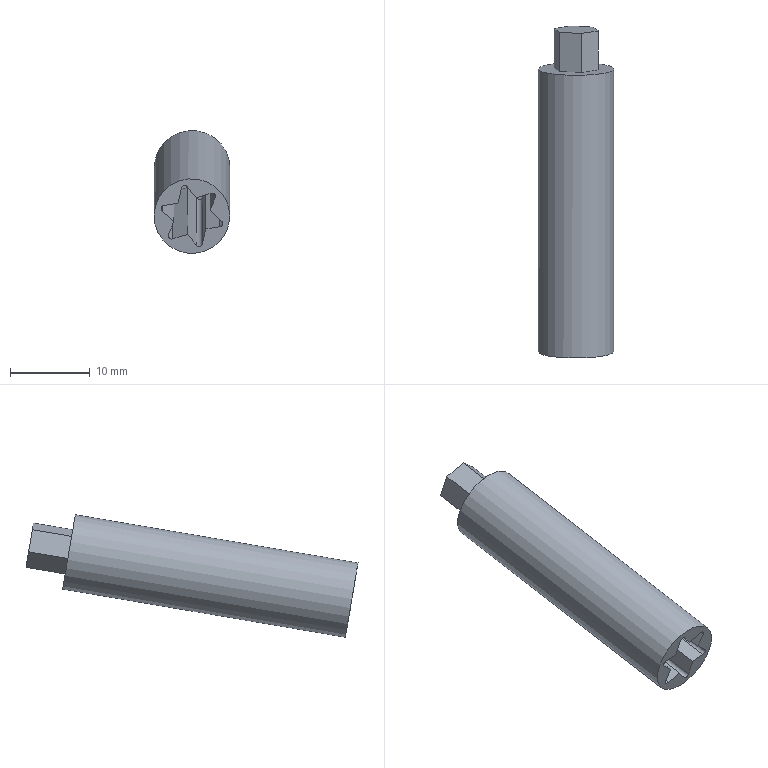Part | STEP file | Dodanie-wyci_gni_cie3 | 1 solid | 31 faces | box 9.523 x 41.689 x 15.416 mm | volume 1560 mm3 | plane 22 | cylinder 9 | commonest cylinder face diameters 0.858 x8 9.5 x1